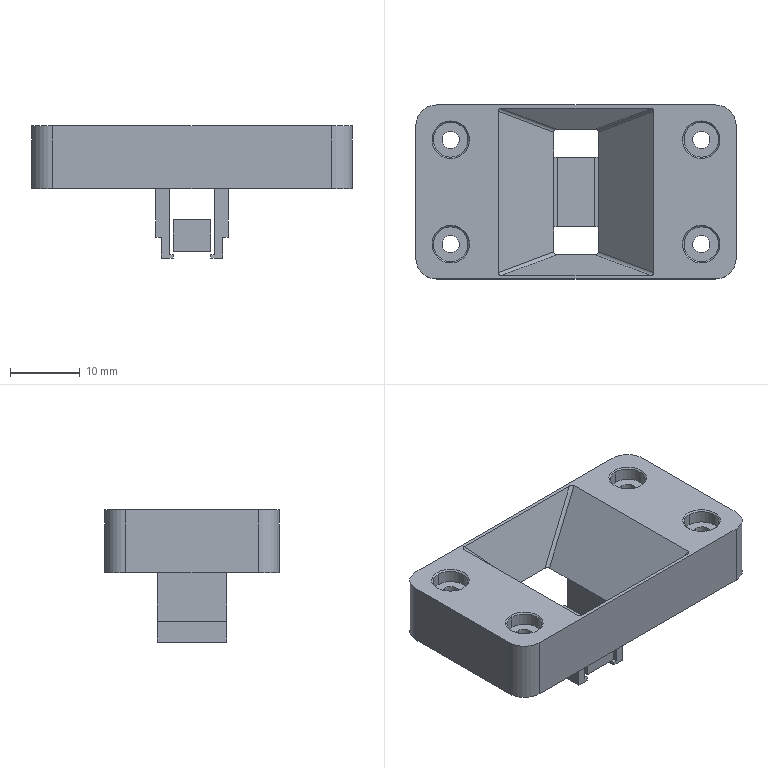NC program | NX | posted with a generic post | part box 46 x 25 x 19 mm
Lines 3678 to 3737 of 3737:
(刀补3 , TOOL : D3)
N7288 T03 M6
N7290 G54
N7292 G17 G0 G90 X-18. Y7.5 S9500 M3
N7294 G43 Z30. H3
N7296 Z0.5
N7298 G41 G94 G1 X-17.996 Y7.4 F1100. D3
N7300 G3 X-17.05 Y7.5 R0.478
N7302 X-17.05 Y7.5 Z-0.5 I-0.95 J0.
N7304 X-17.05 Y7.5 Z-1.5 I-0.95 J0.
N7306 X-18.95 Y7.5 Z-2. I-0.95 J0.
N7308 X-18. Y6.55 R0.95
N7310 X-18.95 Y7.5 R-0.95
N7312 X-18.004 Y7.4 R0.478
N7314 G40
N7316 G1 X-18. Y7.5
N7318 G0 Z30.
N7320 Y-7.5
N7322 Z0.5
N7324 G41 G1 X-17.996 Y-7.6
N7326 G3 X-17.05 Y-7.5 R0.478
N7328 X-17.05 Y-7.5 Z-0.5 I-0.95 J0.
N7330 X-17.05 Y-7.5 Z-1.5 I-0.95 J0.
N7332 X-18.95 Y-7.5 Z-2. I-0.95 J0.
N7334 X-18. Y-8.45 R0.95
N7336 X-18.95 Y-7.5 R-0.95
N7338 X-18.004 Y-7.6 R0.478
N7340 G40
N7342 G1 X-18. Y-7.5
N7344 G0 Z30.
N7346 X18.
N7348 Z0.5
N7350 G41 G1 X18.004 Y-7.6
N7352 G3 X18.95 Y-7.5 R0.478
N7354 X18.95 Y-7.5 Z-0.5 I-0.95 J0.
N7356 X18.95 Y-7.5 Z-1.5 I-0.95 J0.
N7358 X17.05 Y-7.5 Z-2. I-0.95 J0.
N7360 X18. Y-8.45 R0.95
N7362 X17.05 Y-7.5 R-0.95
N7364 X17.996 Y-7.6 R0.478
N7366 G40
N7368 G1 X18. Y-7.5
N7370 G0 Z30.
N7372 Y7.5
N7374 Z0.5
N7376 G41 G1 X18.004 Y7.4
N7378 G3 X18.95 Y7.5 R0.478
N7380 X18.95 Y7.5 Z-0.5 I-0.95 J0.
N7382 X18.95 Y7.5 Z-1.5 I-0.95 J0.
N7384 X17.05 Y7.5 Z-2. I-0.95 J0.
N7386 X18. Y6.55 R0.95
N7388 X17.05 Y7.5 R-0.95
N7390 X17.996 Y7.4 R0.478
N7392 G40
N7394 G1 X18. Y7.5
N7396 G0 Z30.
N7398 M5
N7400 M2